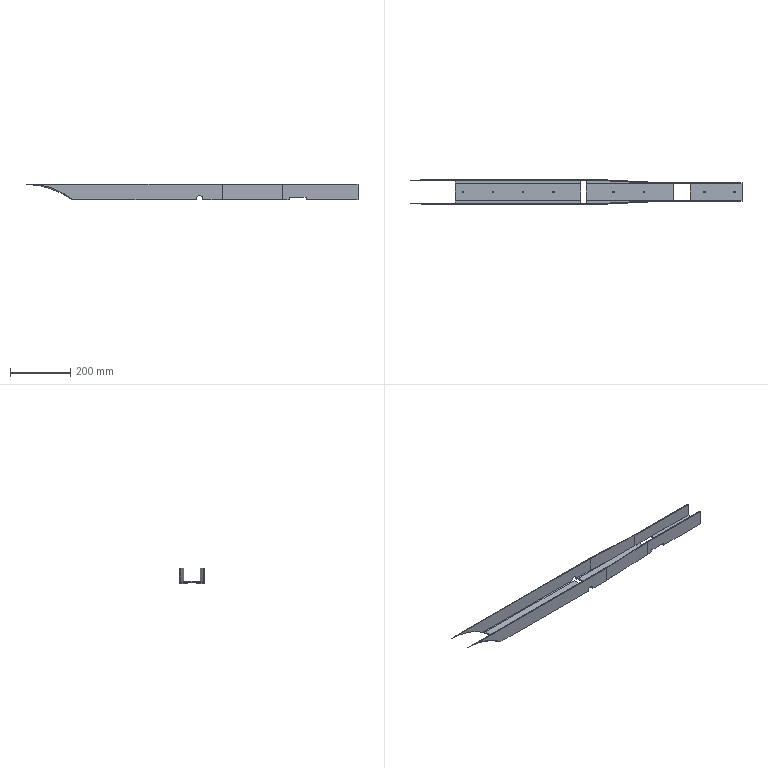Part | SolidWorks | features BaseBody 1 | 1 solid | 77 faces | box 1100 x 80 x 50 mm | volume 533564 mm3 | plane 58 | cylinder 17 | torus 2 | commonest cylinder face diameters 5 x16 22 x1